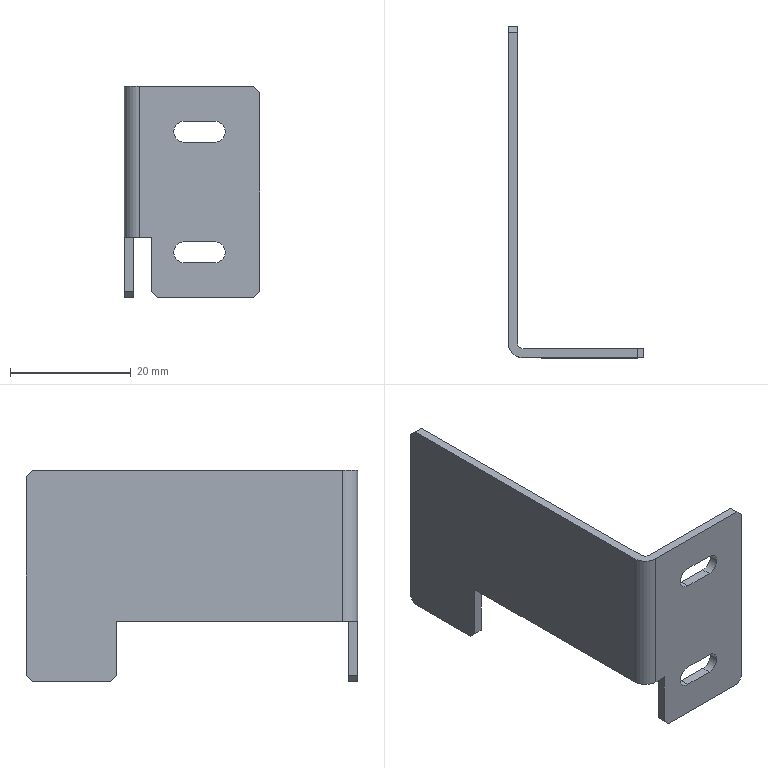Part | SolidWorks | features BaseBody 1 | 1 solid | 28 faces | box 22.5 x 55 x 35 mm | volume 3231 mm3 | plane 22 | cylinder 6 | commonest cylinder face diameters 3.5 x4 2 x1 5 x1
STEP:
#1=CARTESIAN_POINT('',(9.,-1.5,-17.5));
#2=VERTEX_POINT('',#1);
#3=CARTESIAN_POINT('',(10.,-1.5,-16.5));
#4=VERTEX_POINT('',#3);
#5=CARTESIAN_POINT('',(10.,-1.5,-16.5));
#6=DIRECTION('',(0.7071,0.,0.7071));
#7=VECTOR('',#6,1000.);
#8=LINE('',#5,#7);
#9=EDGE_CURVE('',#2,#4,#8,.T.);
#10=ORIENTED_EDGE('',*,*,#9,.F.);
#11=CARTESIAN_POINT('',(9.,0.,-17.5));
#12=VERTEX_POINT('',#11);
#13=CARTESIAN_POINT('',(9.,-1.5,-17.5));
#14=DIRECTION('',(0.,-1.,0.));
#15=VECTOR('',#14,1000.);
#16=LINE('',#13,#15);
#17=EDGE_CURVE('',#12,#2,#16,.T.);
#18=ORIENTED_EDGE('',*,*,#17,.F.);
#19=CARTESIAN_POINT('',(10.,0.,-16.5));
#20=VERTEX_POINT('',#19);
#21=CARTESIAN_POINT('',(13.25,0.,-13.25));
#22=DIRECTION('',(-0.7071,0.,-0.7071));
#23=VECTOR('',#22,1000.);
#24=LINE('',#21,#23);
#25=EDGE_CURVE('',#20,#12,#24,.T.);
#26=ORIENTED_EDGE('',*,*,#25,.F.);
#27=CARTESIAN_POINT('',(10.,-1.5,-16.5));
#28=DIRECTION('',(0.,1.,0.));
#29=VECTOR('',#28,1000.);
#30=LINE('',#27,#29);
#31=EDGE_CURVE('',#4,#20,#30,.T.);
#32=ORIENTED_EDGE('',*,*,#31,.F.);
#33=EDGE_LOOP('',(#10,#18,#26,#32));
#34=FACE_OUTER_BOUND('',#33,.T.);
#35=CARTESIAN_POINT('',(10.,-1.5,-16.5));
#36=DIRECTION('',(-0.7071,0.,0.7071));
#37=DIRECTION('',(0.,1.,0.));
#38=AXIS2_PLACEMENT_3D('',#35,#36,#37);
#39=PLANE('',#38);
#40=ADVANCED_FACE('',(#34),#39,.F.);
#41=CARTESIAN_POINT('',(10.,-1.5,16.5));
#42=VERTEX_POINT('',#41);
#43=CARTESIAN_POINT('',(9.,-1.5,17.5));
#44=VERTEX_POINT('',#43);
#45=CARTESIAN_POINT('',(9.,-1.5,17.5));
#46=DIRECTION('',(-0.7071,0.,0.7071));
#47=VECTOR('',#46,1000.);
#48=LINE('',#45,#47);
#49=EDGE_CURVE('',#42,#44,#48,.T.);
#50=ORIENTED_EDGE('',*,*,#49,.F.);
#51=CARTESIAN_POINT('',(10.,0.,16.5));
#52=VERTEX_POINT('',#51);
#53=CARTESIAN_POINT('',(10.,-1.5,16.5));
#54=DIRECTION('',(0.,-1.,0.));
#55=VECTOR('',#54,1000.);
#56=LINE('',#53,#55);
#57=EDGE_CURVE('',#52,#42,#56,.T.);
#58=ORIENTED_EDGE('',*,*,#57,.F.);
#59=CARTESIAN_POINT('',(9.,0.,17.5));
#60=VERTEX_POINT('',#59);
#61=CARTESIAN_POINT('',(13.25,0.,13.25));
#62=DIRECTION('',(0.7071,0.,-0.7071));
#63=VECTOR('',#62,1000.);
#64=LINE('',#61,#63);
#65=EDGE_CURVE('',#60,#52,#64,.T.);
#66=ORIENTED_EDGE('',*,*,#65,.F.);
#67=CARTESIAN_POINT('',(9.,-1.5,17.5));
#68=DIRECTION('',(0.,1.,0.));
#69=VECTOR('',#68,1000.);
#70=LINE('',#67,#69);
#71=EDGE_CURVE('',#44,#60,#70,.T.);
#72=ORIENTED_EDGE('',*,*,#71,.F.);
#73=EDGE_LOOP('',(#50,#58,#66,#72));
#74=FACE_OUTER_BOUND('',#73,.T.);
#75=CARTESIAN_POINT('',(9.,-1.5,17.5));
#76=DIRECTION('',(-0.7071,0.,-0.7071));
#77=DIRECTION('',(-0.7071,0.,0.7071));
#78=AXIS2_PLACEMENT_3D('',#75,#76,#77);
#79=PLANE('',#78);
#80=ADVANCED_FACE('',(#74),#79,.F.);
#81=CARTESIAN_POINT('',(-8.,-1.5,-16.5));
#82=VERTEX_POINT('',#81);
#83=CARTESIAN_POINT('',(-7.,-1.5,-17.5));
#84=VERTEX_POINT('',#83);
#85=CARTESIAN_POINT('',(-7.,-1.5,-17.5));
#86=DIRECTION('',(0.7071,0.,-0.7071));
#87=VECTOR('',#86,1000.);
#88=LINE('',#85,#87);
#89=EDGE_CURVE('',#82,#84,#88,.T.);
#90=ORIENTED_EDGE('',*,*,#89,.F.);
#91=CARTESIAN_POINT('',(-8.,0.,-16.5));
#92=VERTEX_POINT('',#91);
#93=CARTESIAN_POINT('',(-8.,0.,-16.5));
#94=DIRECTION('',(0.,-1.,0.));
#95=VECTOR('',#94,1000.);
#96=LINE('',#93,#95);
#97=EDGE_CURVE('',#92,#82,#96,.T.);
#98=ORIENTED_EDGE('',*,*,#97,.F.);
#99=CARTESIAN_POINT('',(-7.,0.,-17.5));
#100=VERTEX_POINT('',#99);
#101=CARTESIAN_POINT('',(-12.25,0.,-12.25));
#102=DIRECTION('',(-0.7071,0.,0.7071));
#103=VECTOR('',#102,1000.);
#104=LINE('',#101,#103);
#105=EDGE_CURVE('',#100,#92,#104,.T.);
#106=ORIENTED_EDGE('',*,*,#105,.F.);
#107=CARTESIAN_POINT('',(-7.,-1.5,-17.5));
#108=DIRECTION('',(0.,1.,0.));
#109=VECTOR('',#108,1000.);
#110=LINE('',#107,#109);
#111=EDGE_CURVE('',#84,#100,#110,.T.);
#112=ORIENTED_EDGE('',*,*,#111,.F.);
#113=EDGE_LOOP('',(#90,#98,#106,#112));
#114=FACE_OUTER_BOUND('',#113,.T.);
#115=CARTESIAN_POINT('',(-7.,-1.5,-17.5));
#116=DIRECTION('',(0.7071,0.,0.7071));
#117=DIRECTION('',(0.,-1.,0.));
#118=AXIS2_PLACEMENT_3D('',#115,#116,#117);
#119=PLANE('',#118);
#120=ADVANCED_FACE('',(#114),#119,.F.);
#121=CARTESIAN_POINT('',(-12.5,53.5,-16.5));
#122=VERTEX_POINT('',#121);
#123=CARTESIAN_POINT('',(-12.5,52.5,-17.5));
#124=VERTEX_POINT('',#123);
#125=CARTESIAN_POINT('',(-12.5,52.5,-17.5));
#126=DIRECTION('',(0.,-0.7071,-0.7071));
#127=VECTOR('',#126,1000.);
#128=LINE('',#125,#127);
#129=EDGE_CURVE('',#122,#124,#128,.T.);
#130=ORIENTED_EDGE('',*,*,#129,.F.);
#131=CARTESIAN_POINT('',(-11.,53.5,-16.5));
#132=VERTEX_POINT('',#131);
#133=CARTESIAN_POINT('',(-12.5,53.5,-16.5));
#134=DIRECTION('',(-1.,0.,0.));
#135=VECTOR('',#134,1000.);
#136=LINE('',#133,#135);
#137=EDGE_CURVE('',#132,#122,#136,.T.);
#138=ORIENTED_EDGE('',*,*,#137,.F.);
#139=CARTESIAN_POINT('',(-11.,52.5,-17.5));
#140=VERTEX_POINT('',#139);
#141=CARTESIAN_POINT('',(-11.,35.,-35.));
#142=DIRECTION('',(0.,0.7071,0.7071));
#143=VECTOR('',#142,1000.);
#144=LINE('',#141,#143);
#145=EDGE_CURVE('',#140,#132,#144,.T.);
#146=ORIENTED_EDGE('',*,*,#145,.F.);
#147=CARTESIAN_POINT('',(-12.5,52.5,-17.5));
#148=DIRECTION('',(1.,0.,0.));
#149=VECTOR('',#148,1000.);
#150=LINE('',#147,#149);
#151=EDGE_CURVE('',#124,#140,#150,.T.);
#152=ORIENTED_EDGE('',*,*,#151,.F.);
#153=EDGE_LOOP('',(#130,#138,#146,#152));
#154=FACE_OUTER_BOUND('',#153,.T.);
#155=CARTESIAN_POINT('',(-12.5,52.5,-17.5));
#156=DIRECTION('',(0.,-0.7071,0.7071));
#157=DIRECTION('',(-1.,0.,0.));
#158=AXIS2_PLACEMENT_3D('',#155,#156,#157);
#159=PLANE('',#158);
#160=ADVANCED_FACE('',(#154),#159,.F.);
#161=CARTESIAN_POINT('',(-12.5,39.5,-17.5));
#162=VERTEX_POINT('',#161);
#163=CARTESIAN_POINT('',(-12.5,38.5,-16.5));
#164=VERTEX_POINT('',#163);
#165=CARTESIAN_POINT('',(-12.5,38.5,-16.5));
#166=DIRECTION('',(0.,-0.7071,0.7071));
#167=VECTOR('',#166,1000.);
#168=LINE('',#165,#167);
#169=EDGE_CURVE('',#162,#164,#168,.T.);
#170=ORIENTED_EDGE('',*,*,#169,.F.);
#171=CARTESIAN_POINT('',(-11.,39.5,-17.5));
#172=VERTEX_POINT('',#171);
#173=CARTESIAN_POINT('',(-12.5,39.5,-17.5));
#174=DIRECTION('',(-1.,0.,0.));
#175=VECTOR('',#174,1000.);
#176=LINE('',#173,#175);
#177=EDGE_CURVE('',#172,#162,#176,.T.);
#178=ORIENTED_EDGE('',*,*,#177,.F.);
#179=CARTESIAN_POINT('',(-11.,38.5,-16.5));
#180=VERTEX_POINT('',#179);
#181=CARTESIAN_POINT('',(-11.,11.,11.));
#182=DIRECTION('',(0.,0.7071,-0.7071));
#183=VECTOR('',#182,1000.);
#184=LINE('',#181,#183);
#185=EDGE_CURVE('',#180,#172,#184,.T.);
#186=ORIENTED_EDGE('',*,*,#185,.F.);
#187=CARTESIAN_POINT('',(-14.,38.5,-16.5));
#188=DIRECTION('',(1.,0.,0.));
#189=VECTOR('',#188,1000.);
#190=LINE('',#187,#189);
#191=EDGE_CURVE('',#164,#180,#190,.T.);
#192=ORIENTED_EDGE('',*,*,#191,.F.);
#193=EDGE_LOOP('',(#170,#178,#186,#192));
#194=FACE_OUTER_BOUND('',#193,.T.);
#195=CARTESIAN_POINT('',(-14.,38.5,-16.5));
#196=DIRECTION('',(0.,0.7071,0.7071));
#197=DIRECTION('',(1.,0.,0.));
#198=AXIS2_PLACEMENT_3D('',#195,#196,#197);
#199=PLANE('',#198);
#200=ADVANCED_FACE('',(#194),#199,.F.);
#201=CARTESIAN_POINT('',(-12.5,52.5,17.5));
#202=VERTEX_POINT('',#201);
#203=CARTESIAN_POINT('',(-12.5,53.5,16.5));
#204=VERTEX_POINT('',#203);
#205=CARTESIAN_POINT('',(-12.5,53.5,16.5));
#206=DIRECTION('',(0.,0.7071,-0.7071));
#207=VECTOR('',#206,1000.);
#208=LINE('',#205,#207);
#209=EDGE_CURVE('',#202,#204,#208,.T.);
#210=ORIENTED_EDGE('',*,*,#209,.F.);
#211=CARTESIAN_POINT('',(-11.,52.5,17.5));
#212=VERTEX_POINT('',#211);
#213=CARTESIAN_POINT('',(-12.5,52.5,17.5));
#214=DIRECTION('',(-1.,0.,0.));
#215=VECTOR('',#214,1000.);
#216=LINE('',#213,#215);
#217=EDGE_CURVE('',#212,#202,#216,.T.);
#218=ORIENTED_EDGE('',*,*,#217,.F.);
#219=CARTESIAN_POINT('',(-11.,53.5,16.5));
#220=VERTEX_POINT('',#219);
#221=CARTESIAN_POINT('',(-11.,35.,35.));
#222=DIRECTION('',(0.,-0.7071,0.7071));
#223=VECTOR('',#222,1000.);
#224=LINE('',#221,#223);
#225=EDGE_CURVE('',#220,#212,#224,.T.);
#226=ORIENTED_EDGE('',*,*,#225,.F.);
#227=CARTESIAN_POINT('',(-12.5,53.5,16.5));
#228=DIRECTION('',(1.,0.,0.));
#229=VECTOR('',#228,1000.);
#230=LINE('',#227,#229);
#231=EDGE_CURVE('',#204,#220,#230,.T.);
#232=ORIENTED_EDGE('',*,*,#231,.F.);
#233=EDGE_LOOP('',(#210,#218,#226,#232));
#234=FACE_OUTER_BOUND('',#233,.T.);
#235=CARTESIAN_POINT('',(-12.5,53.5,16.5));
#236=DIRECTION('',(0.,-0.7071,-0.7071));
#237=DIRECTION('',(0.,-0.7071,0.7071));
#238=AXIS2_PLACEMENT_3D('',#235,#236,#237);
#239=PLANE('',#238);
#240=ADVANCED_FACE('',(#234),#239,.F.);
#241=CARTESIAN_POINT('',(-12.5,38.5,-7.5));
#242=VERTEX_POINT('',#241);
#243=CARTESIAN_POINT('',(-12.5,38.5,0.));
#244=DIRECTION('',(0.,0.,1.));
#245=VECTOR('',#244,1000.);
#246=LINE('',#243,#245);
#247=EDGE_CURVE('',#164,#242,#246,.T.);
#248=ORIENTED_EDGE('',*,*,#247,.F.);
#249=ORIENTED_EDGE('',*,*,#191,.T.);
#250=CARTESIAN_POINT('',(-11.,38.5,-7.5));
#251=VERTEX_POINT('',#250);
#252=CARTESIAN_POINT('',(-11.,38.5,0.));
#253=DIRECTION('',(0.,0.,1.));
#254=VECTOR('',#253,1000.);
#255=LINE('',#252,#254);
#256=EDGE_CURVE('',#180,#251,#255,.T.);
#257=ORIENTED_EDGE('',*,*,#256,.T.);
#258=CARTESIAN_POINT('',(-14.,38.5,-7.5));
#259=DIRECTION('',(1.,0.,0.));
#260=VECTOR('',#259,1000.);
#261=LINE('',#258,#260);
#262=EDGE_CURVE('',#242,#251,#261,.T.);
#263=ORIENTED_EDGE('',*,*,#262,.F.);
#264=EDGE_LOOP('',(#248,#249,#257,#263));
#265=FACE_OUTER_BOUND('',#264,.T.);
#266=CARTESIAN_POINT('',(-14.,38.5,-17.5));
#267=DIRECTION('',(0.,1.,0.));
#268=DIRECTION('',(1.,0.,0.));
#269=AXIS2_PLACEMENT_3D('',#266,#267,#268);
#270=PLANE('',#269);
#271=ADVANCED_FACE('',(#265),#270,.F.);
#272=CARTESIAN_POINT('',(-10.,-1.5,-7.5));
#273=VERTEX_POINT('',#272);
#274=CARTESIAN_POINT('',(-12.5,1.,-7.5));
#275=VERTEX_POINT('',#274);
#276=CARTESIAN_POINT('',(-10.,1.,-7.5));
#277=DIRECTION('',(0.,0.,-1.));
#278=DIRECTION('',(0.,-1.,0.));
#279=AXIS2_PLACEMENT_3D('',#276,#277,#278);
#280=CIRCLE('',#279,2.5);
#281=EDGE_CURVE('',#273,#275,#280,.T.);
#282=ORIENTED_EDGE('',*,*,#281,.T.);
#283=CARTESIAN_POINT('',(-12.5,0.,-7.5));
#284=DIRECTION('',(0.,-1.,0.));
#285=VECTOR('',#284,1000.);
#286=LINE('',#283,#285);
#287=EDGE_CURVE('',#242,#275,#286,.T.);
#288=ORIENTED_EDGE('',*,*,#287,.F.);
#289=ORIENTED_EDGE('',*,*,#262,.T.);
#290=CARTESIAN_POINT('',(-11.,1.,-7.5));
#291=VERTEX_POINT('',#290);
#292=CARTESIAN_POINT('',(-11.,0.,-7.5));
#293=DIRECTION('',(0.,-1.,0.));
#294=VECTOR('',#293,1000.);
#295=LINE('',#292,#294);
#296=EDGE_CURVE('',#251,#291,#295,.T.);
#297=ORIENTED_EDGE('',*,*,#296,.T.);
#298=CARTESIAN_POINT('',(-10.,0.,-7.5));
#299=VERTEX_POINT('',#298);
#300=CARTESIAN_POINT('',(-10.,1.,-7.5));
#301=DIRECTION('',(0.,0.,-1.));
#302=DIRECTION('',(0.,-1.,0.));
#303=AXIS2_PLACEMENT_3D('',#300,#301,#302);
#304=CIRCLE('',#303,1.);
#305=EDGE_CURVE('',#299,#291,#304,.T.);
#306=ORIENTED_EDGE('',*,*,#305,.F.);
#307=CARTESIAN_POINT('',(-8.,0.,-7.5));
#308=VERTEX_POINT('',#307);
#309=CARTESIAN_POINT('',(0.,0.,-7.5));
#310=DIRECTION('',(1.,0.,0.));
#311=VECTOR('',#310,1000.);
#312=LINE('',#309,#311);
#313=EDGE_CURVE('',#299,#308,#312,.T.);
#314=ORIENTED_EDGE('',*,*,#313,.T.);
#315=CARTESIAN_POINT('',(-8.,-1.5,-7.5));
#316=VERTEX_POINT('',#315);
#317=CARTESIAN_POINT('',(-8.,38.5,-7.5));
#318=DIRECTION('',(0.,-1.,0.));
#319=VECTOR('',#318,1000.);
#320=LINE('',#317,#319);
#321=EDGE_CURVE('',#308,#316,#320,.T.);
#322=ORIENTED_EDGE('',*,*,#321,.T.);
#323=CARTESIAN_POINT('',(0.,-1.5,-7.5));
#324=DIRECTION('',(1.,0.,0.));
#325=VECTOR('',#324,1000.);
#326=LINE('',#323,#325);
#327=EDGE_CURVE('',#273,#316,#326,.T.);
#328=ORIENTED_EDGE('',*,*,#327,.F.);
#329=EDGE_LOOP('',(#282,#288,#289,#297,#306,#314,#322,#328));
#330=FACE_OUTER_BOUND('',#329,.T.);
#331=CARTESIAN_POINT('',(-14.,38.5,-7.5));
#332=DIRECTION('',(0.,0.,1.));
#333=DIRECTION('',(0.,-1.,0.));
#334=AXIS2_PLACEMENT_3D('',#331,#332,#333);
#335=PLANE('',#334);
#336=ADVANCED_FACE('',(#330),#335,.F.);
#337=CARTESIAN_POINT('',(-8.,0.,0.));
#338=DIRECTION('',(0.,0.,1.));
#339=VECTOR('',#338,1000.);
#340=LINE('',#337,#339);
#341=EDGE_CURVE('',#92,#308,#340,.T.);
#342=ORIENTED_EDGE('',*,*,#341,.F.);
#343=ORIENTED_EDGE('',*,*,#97,.T.);
#344=CARTESIAN_POINT('',(-8.,-1.5,0.));
#345=DIRECTION('',(0.,0.,1.));
#346=VECTOR('',#345,1000.);
#347=LINE('',#344,#346);
#348=EDGE_CURVE('',#82,#316,#347,.T.);
#349=ORIENTED_EDGE('',*,*,#348,.T.);
#350=ORIENTED_EDGE('',*,*,#321,.F.);
#351=EDGE_LOOP('',(#342,#343,#349,#350));
#352=FACE_OUTER_BOUND('',#351,.T.);
#353=CARTESIAN_POINT('',(-8.,0.,0.));
#354=DIRECTION('',(-1.,0.,0.));
#355=DIRECTION('',(0.,1.,0.));
#356=AXIS2_PLACEMENT_3D('',#353,#354,#355);
#357=PLANE('',#356);
#358=ADVANCED_FACE('',(#352),#357,.T.);
#359=CARTESIAN_POINT('',(2.5,0.,11.75));
#360=VERTEX_POINT('',#359);
#361=CARTESIAN_POINT('',(2.5,0.,8.25));
#362=VERTEX_POINT('',#361);
#363=CARTESIAN_POINT('',(2.5,0.,10.));
#364=DIRECTION('',(0.,1.,0.));
#365=DIRECTION('',(0.,0.,1.));
#366=AXIS2_PLACEMENT_3D('',#363,#364,#365);
#367=CIRCLE('',#366,1.75);
#368=EDGE_CURVE('',#360,#362,#367,.T.);
#369=ORIENTED_EDGE('',*,*,#368,.T.);
#370=CARTESIAN_POINT('',(2.5,-1.5,8.25));
#371=VERTEX_POINT('',#370);
#372=CARTESIAN_POINT('',(2.5,8.5,8.25));
#373=DIRECTION('',(0.,-1.,0.));
#374=VECTOR('',#373,1000.);
#375=LINE('',#372,#374);
#376=EDGE_CURVE('',#362,#371,#375,.T.);
#377=ORIENTED_EDGE('',*,*,#376,.T.);
#378=CARTESIAN_POINT('',(2.5,-1.5,11.75));
#379=VERTEX_POINT('',#378);
#380=CARTESIAN_POINT('',(2.5,-1.5,10.));
#381=DIRECTION('',(0.,-1.,0.));
#382=DIRECTION('',(0.,0.,-1.));
#383=AXIS2_PLACEMENT_3D('',#380,#381,#382);
#384=CIRCLE('',#383,1.75);
#385=EDGE_CURVE('',#371,#379,#384,.T.);
#386=ORIENTED_EDGE('',*,*,#385,.T.);
#387=CARTESIAN_POINT('',(2.5,8.5,11.75));
#388=DIRECTION('',(0.,-1.,0.));
#389=VECTOR('',#388,1000.);
#390=LINE('',#387,#389);
#391=EDGE_CURVE('',#360,#379,#390,.T.);
#392=ORIENTED_EDGE('',*,*,#391,.F.);
#393=EDGE_LOOP('',(#369,#377,#386,#392));
#394=FACE_OUTER_BOUND('',#393,.T.);
#395=CARTESIAN_POINT('',(2.5,8.5,10.));
#396=DIRECTION('',(0.,-1.,0.));
#397=DIRECTION('',(0.,0.,-1.));
#398=AXIS2_PLACEMENT_3D('',#395,#396,#397);
#399=CYLINDRICAL_SURFACE('',#398,1.75);
#400=ADVANCED_FACE('',(#394),#399,.F.);
#401=CARTESIAN_POINT('',(-2.5,0.,8.25));
#402=VERTEX_POINT('',#401);
#403=CARTESIAN_POINT('',(-2.5,0.,11.75));
#404=VERTEX_POINT('',#403);
#405=CARTESIAN_POINT('',(-2.5,0.,10.));
#406=DIRECTION('',(0.,1.,0.));
#407=DIRECTION('',(0.,0.,1.));
#408=AXIS2_PLACEMENT_3D('',#405,#406,#407);
#409=CIRCLE('',#408,1.75);
#410=EDGE_CURVE('',#402,#404,#409,.T.);
#411=ORIENTED_EDGE('',*,*,#410,.T.);
#412=CARTESIAN_POINT('',(-2.5,-1.5,11.75));
#413=VERTEX_POINT('',#412);
#414=CARTESIAN_POINT('',(-2.5,8.5,11.75));
#415=DIRECTION('',(0.,-1.,0.));
#416=VECTOR('',#415,1000.);
#417=LINE('',#414,#416);
#418=EDGE_CURVE('',#404,#413,#417,.T.);
#419=ORIENTED_EDGE('',*,*,#418,.T.);
#420=CARTESIAN_POINT('',(-2.5,-1.5,8.25));
#421=VERTEX_POINT('',#420);
#422=CARTESIAN_POINT('',(-2.5,-1.5,10.));
#423=DIRECTION('',(0.,-1.,0.));
#424=DIRECTION('',(0.,0.,-1.));
#425=AXIS2_PLACEMENT_3D('',#422,#423,#424);
#426=CIRCLE('',#425,1.75);
#427=EDGE_CURVE('',#413,#421,#426,.T.);
#428=ORIENTED_EDGE('',*,*,#427,.T.);
#429=CARTESIAN_POINT('',(-2.5,8.5,8.25));
#430=DIRECTION('',(0.,-1.,0.));
#431=VECTOR('',#430,1000.);
#432=LINE('',#429,#431);
#433=EDGE_CURVE('',#402,#421,#432,.T.);
#434=ORIENTED_EDGE('',*,*,#433,.F.);
#435=EDGE_LOOP('',(#411,#419,#428,#434));
#436=FACE_OUTER_BOUND('',#435,.T.);
#437=CARTESIAN_POINT('',(-2.5,8.5,10.));
#438=DIRECTION('',(0.,-1.,0.));
#439=DIRECTION('',(0.,0.,-1.));
#440=AXIS2_PLACEMENT_3D('',#437,#438,#439);
#441=CYLINDRICAL_SURFACE('',#440,1.75);
#442=ADVANCED_FACE('',(#436),#441,.F.);
#443=CARTESIAN_POINT('',(0.,0.,8.25));
#444=DIRECTION('',(-1.,0.,0.));
#445=VECTOR('',#444,1000.);
#446=LINE('',#443,#445);
#447=EDGE_CURVE('',#362,#402,#446,.T.);
#448=ORIENTED_EDGE('',*,*,#447,.T.);
#449=ORIENTED_EDGE('',*,*,#433,.T.);
#450=CARTESIAN_POINT('',(-2.5,-1.5,8.25));
#451=DIRECTION('',(1.,0.,0.));
#452=VECTOR('',#451,1000.);
#453=LINE('',#450,#452);
#454=EDGE_CURVE('',#421,#371,#453,.T.);
#455=ORIENTED_EDGE('',*,*,#454,.T.);
#456=ORIENTED_EDGE('',*,*,#376,.F.);
#457=EDGE_LOOP('',(#448,#449,#455,#456));
#458=FACE_OUTER_BOUND('',#457,.T.);
#459=CARTESIAN_POINT('',(-2.5,8.5,8.25));
#460=DIRECTION('',(0.,0.,-1.));
#461=DIRECTION('',(0.,-1.,0.));
#462=AXIS2_PLACEMENT_3D('',#459,#460,#461);
#463=PLANE('',#462);
#464=ADVANCED_FACE('',(#458),#463,.F.);
#465=CARTESIAN_POINT('',(0.,0.,11.75));
#466=DIRECTION('',(1.,0.,0.));
#467=VECTOR('',#466,1000.);
#468=LINE('',#465,#467);
#469=EDGE_CURVE('',#404,#360,#468,.T.);
#470=ORIENTED_EDGE('',*,*,#469,.T.);
#471=ORIENTED_EDGE('',*,*,#391,.T.);
#472=CARTESIAN_POINT('',(-2.5,-1.5,11.75));
#473=DIRECTION('',(-1.,0.,0.));
#474=VECTOR('',#473,1000.);
#475=LINE('',#472,#474);
#476=EDGE_CURVE('',#379,#413,#475,.T.);
#477=ORIENTED_EDGE('',*,*,#476,.T.);
#478=ORIENTED_EDGE('',*,*,#418,.F.);
#479=EDGE_LOOP('',(#470,#471,#477,#478));
#480=FACE_OUTER_BOUND('',#479,.T.);
#481=CARTESIAN_POINT('',(-2.5,8.5,11.75));
#482=DIRECTION('',(0.,0.,1.));
#483=DIRECTION('',(1.,0.,0.));
#484=AXIS2_PLACEMENT_3D('',#481,#482,#483);
#485=PLANE('',#484);
#486=ADVANCED_FACE('',(#480),#485,.F.);
#487=CARTESIAN_POINT('',(2.5,0.,-8.25));
#488=VERTEX_POINT('',#487);
#489=CARTESIAN_POINT('',(2.5,0.,-11.75));
#490=VERTEX_POINT('',#489);
#491=CARTESIAN_POINT('',(2.5,0.,-10.));
#492=DIRECTION('',(0.,1.,0.));
#493=DIRECTION('',(0.,0.,1.));
#494=AXIS2_PLACEMENT_3D('',#491,#492,#493);
#495=CIRCLE('',#494,1.75);
#496=EDGE_CURVE('',#488,#490,#495,.T.);
#497=ORIENTED_EDGE('',*,*,#496,.T.);
#498=CARTESIAN_POINT('',(2.5,-1.5,-11.75));
#499=VERTEX_POINT('',#498);
#500=CARTESIAN_POINT('',(2.5,8.5,-11.75));
#501=DIRECTION('',(0.,-1.,0.));
#502=VECTOR('',#501,1000.);
#503=LINE('',#500,#502);
#504=EDGE_CURVE('',#490,#499,#503,.T.);
#505=ORIENTED_EDGE('',*,*,#504,.T.);
#506=CARTESIAN_POINT('',(2.5,-1.5,-8.25));
#507=VERTEX_POINT('',#506);
#508=CARTESIAN_POINT('',(2.5,-1.5,-10.));
#509=DIRECTION('',(0.,-1.,0.));
#510=DIRECTION('',(0.,0.,-1.));
#511=AXIS2_PLACEMENT_3D('',#508,#509,#510);
#512=CIRCLE('',#511,1.75);
#513=EDGE_CURVE('',#499,#507,#512,.T.);
#514=ORIENTED_EDGE('',*,*,#513,.T.);
#515=CARTESIAN_POINT('',(2.5,8.5,-8.25));
#516=DIRECTION('',(0.,-1.,0.));
#517=VECTOR('',#516,1000.);
#518=LINE('',#515,#517);
#519=EDGE_CURVE('',#488,#507,#518,.T.);
#520=ORIENTED_EDGE('',*,*,#519,.F.);
#521=EDGE_LOOP('',(#497,#505,#514,#520));
#522=FACE_OUTER_BOUND('',#521,.T.);
#523=CARTESIAN_POINT('',(2.5,8.5,-10.));
#524=DIRECTION('',(0.,-1.,0.));
#525=DIRECTION('',(0.,0.,-1.));
#526=AXIS2_PLACEMENT_3D('',#523,#524,#525);
#527=CYLINDRICAL_SURFACE('',#526,1.75);
#528=ADVANCED_FACE('',(#522),#527,.F.);
#529=CARTESIAN_POINT('',(-2.5,0.,-11.75));
#530=VERTEX_POINT('',#529);
#531=CARTESIAN_POINT('',(-2.5,0.,-8.25));
#532=VERTEX_POINT('',#531);
#533=CARTESIAN_POINT('',(-2.5,0.,-10.));
#534=DIRECTION('',(0.,1.,0.));
#535=DIRECTION('',(0.,0.,1.));
#536=AXIS2_PLACEMENT_3D('',#533,#534,#535);
#537=CIRCLE('',#536,1.75);
#538=EDGE_CURVE('',#530,#532,#537,.T.);
#539=ORIENTED_EDGE('',*,*,#538,.T.);
#540=CARTESIAN_POINT('',(-2.5,-1.5,-8.25));
#541=VERTEX_POINT('',#540);
#542=CARTESIAN_POINT('',(-2.5,8.5,-8.25));
#543=DIRECTION('',(0.,-1.,0.));
#544=VECTOR('',#543,1000.);
#545=LINE('',#542,#544);
#546=EDGE_CURVE('',#532,#541,#545,.T.);
#547=ORIENTED_EDGE('',*,*,#546,.T.);
#548=CARTESIAN_POINT('',(-2.5,-1.5,-11.75));
#549=VERTEX_POINT('',#548);
#550=CARTESIAN_POINT('',(-2.5,-1.5,-10.));
#551=DIRECTION('',(0.,-1.,0.));
#552=DIRECTION('',(0.,0.,-1.));
#553=AXIS2_PLACEMENT_3D('',#550,#551,#552);
#554=CIRCLE('',#553,1.75);
#555=EDGE_CURVE('',#541,#549,#554,.T.);
#556=ORIENTED_EDGE('',*,*,#555,.T.);
#557=CARTESIAN_POINT('',(-2.5,8.5,-11.75));
#558=DIRECTION('',(0.,-1.,0.));
#559=VECTOR('',#558,1000.);
#560=LINE('',#557,#559);
#561=EDGE_CURVE('',#530,#549,#560,.T.);
#562=ORIENTED_EDGE('',*,*,#561,.F.);
#563=EDGE_LOOP('',(#539,#547,#556,#562));
#564=FACE_OUTER_BOUND('',#563,.T.);
#565=CARTESIAN_POINT('',(-2.5,8.5,-10.));
#566=DIRECTION('',(0.,-1.,0.));
#567=DIRECTION('',(0.,0.,-1.));
#568=AXIS2_PLACEMENT_3D('',#565,#566,#567);
#569=CYLINDRICAL_SURFACE('',#568,1.75);
#570=ADVANCED_FACE('',(#564),#569,.F.);
#571=CARTESIAN_POINT('',(0.,0.,-11.75));
#572=DIRECTION('',(-1.,0.,0.));
#573=VECTOR('',#572,1000.);
#574=LINE('',#571,#573);
#575=EDGE_CURVE('',#490,#530,#574,.T.);
#576=ORIENTED_EDGE('',*,*,#575,.T.);
#577=ORIENTED_EDGE('',*,*,#561,.T.);
#578=CARTESIAN_POINT('',(-2.5,-1.5,-11.75));
#579=DIRECTION('',(1.,0.,0.));
#580=VECTOR('',#579,1000.);
#581=LINE('',#578,#580);
#582=EDGE_CURVE('',#549,#499,#581,.T.);
#583=ORIENTED_EDGE('',*,*,#582,.T.);
#584=ORIENTED_EDGE('',*,*,#504,.F.);
#585=EDGE_LOOP('',(#576,#577,#583,#584));
#586=FACE_OUTER_BOUND('',#585,.T.);
#587=CARTESIAN_POINT('',(-2.5,8.5,-11.75));
#588=DIRECTION('',(0.,0.,-1.));
#589=DIRECTION('',(0.,-1.,0.));
#590=AXIS2_PLACEMENT_3D('',#587,#588,#589);
#591=PLANE('',#590);
#592=ADVANCED_FACE('',(#586),#591,.F.);
#593=CARTESIAN_POINT('',(0.,0.,-8.25));
#594=DIRECTION('',(1.,0.,0.));
#595=VECTOR('',#594,1000.);
#596=LINE('',#593,#595);
#597=EDGE_CURVE('',#532,#488,#596,.T.);
#598=ORIENTED_EDGE('',*,*,#597,.T.);
#599=ORIENTED_EDGE('',*,*,#519,.T.);
#600=CARTESIAN_POINT('',(-2.5,-1.5,-8.25));
#601=DIRECTION('',(-1.,0.,0.));
#602=VECTOR('',#601,1000.);
#603=LINE('',#600,#602);
#604=EDGE_CURVE('',#507,#541,#603,.T.);
#605=ORIENTED_EDGE('',*,*,#604,.T.);
#606=ORIENTED_EDGE('',*,*,#546,.F.);
#607=EDGE_LOOP('',(#598,#599,#605,#606));
#608=FACE_OUTER_BOUND('',#607,.T.);
#609=CARTESIAN_POINT('',(-2.5,8.5,-8.25));
#610=DIRECTION('',(0.,0.,1.));
#611=DIRECTION('',(1.,0.,0.));
#612=AXIS2_PLACEMENT_3D('',#609,#610,#611);
#613=PLANE('',#612);
#614=ADVANCED_FACE('',(#608),#613,.F.);
#615=CARTESIAN_POINT('',(-12.5,53.5,0.));
#616=DIRECTION('',(0.,0.,-1.));
#617=VECTOR('',#616,1000.);
#618=LINE('',#615,#617);
#619=EDGE_CURVE('',#204,#122,#618,.T.);
#620=ORIENTED_EDGE('',*,*,#619,.F.);
#621=ORIENTED_EDGE('',*,*,#231,.T.);
#622=CARTESIAN_POINT('',(-11.,53.5,-17.5));
#623=DIRECTION('',(0.,0.,-1.));
#624=VECTOR('',#623,1000.);
#625=LINE('',#622,#624);
#626=EDGE_CURVE('',#220,#132,#625,.T.);
#627=ORIENTED_EDGE('',*,*,#626,.T.);
#628=ORIENTED_EDGE('',*,*,#137,.T.);
#629=EDGE_LOOP('',(#620,#621,#627,#628));
#630=FACE_OUTER_BOUND('',#629,.T.);
#631=CARTESIAN_POINT('',(-12.5,53.5,-17.5));
#632=DIRECTION('',(0.,-1.,0.));
#633=DIRECTION('',(0.,0.,-1.));
#634=AXIS2_PLACEMENT_3D('',#631,#632,#633);
#635=PLANE('',#634);
#636=ADVANCED_FACE('',(#630),#635,.F.);
#637=ORIENTED_EDGE('',*,*,#626,.F.);
#638=ORIENTED_EDGE('',*,*,#225,.T.);
#639=CARTESIAN_POINT('',(-11.,1.,17.5));
#640=VERTEX_POINT('',#639);
#641=CARTESIAN_POINT('',(-11.,53.5,17.5));
#642=DIRECTION('',(0.,1.,0.));
#643=VECTOR('',#642,1000.);
#644=LINE('',#641,#643);
#645=EDGE_CURVE('',#640,#212,#644,.T.);
#646=ORIENTED_EDGE('',*,*,#645,.F.);
#647=CARTESIAN_POINT('',(-11.,1.,-17.5));
#648=DIRECTION('',(0.,0.,1.));
#649=VECTOR('',#648,1000.);
#650=LINE('',#647,#649);
#651=EDGE_CURVE('',#291,#640,#650,.T.);
#652=ORIENTED_EDGE('',*,*,#651,.F.);
#653=ORIENTED_EDGE('',*,*,#296,.F.);
#654=ORIENTED_EDGE('',*,*,#256,.F.);
#655=ORIENTED_EDGE('',*,*,#185,.T.);
#656=CARTESIAN_POINT('',(-11.,0.,-17.5));
#657=DIRECTION('',(0.,-1.,0.));
#658=VECTOR('',#657,1000.);
#659=LINE('',#656,#658);
#660=EDGE_CURVE('',#140,#172,#659,.T.);
#661=ORIENTED_EDGE('',*,*,#660,.F.);
#662=ORIENTED_EDGE('',*,*,#145,.T.);
#663=EDGE_LOOP('',(#637,#638,#646,#652,#653,#654,#655,#661,#662));
#664=FACE_OUTER_BOUND('',#663,.T.);
#665=CARTESIAN_POINT('',(-11.,0.,0.));
#666=DIRECTION('',(1.,0.,0.));
#667=DIRECTION('',(0.,1.,0.));
#668=AXIS2_PLACEMENT_3D('',#665,#666,#667);
#669=PLANE('',#668);
#670=ADVANCED_FACE('',(#664),#669,.T.);
#671=CARTESIAN_POINT('',(-12.5,1.,17.5));
#672=VERTEX_POINT('',#671);
#673=CARTESIAN_POINT('',(-12.5,0.,17.5));
#674=DIRECTION('',(0.,1.,0.));
#675=VECTOR('',#674,1000.);
#676=LINE('',#673,#675);
#677=EDGE_CURVE('',#672,#202,#676,.T.);
#678=ORIENTED_EDGE('',*,*,#677,.T.);
#679=ORIENTED_EDGE('',*,*,#209,.T.);
#680=ORIENTED_EDGE('',*,*,#619,.T.);
#681=ORIENTED_EDGE('',*,*,#129,.T.);
#682=CARTESIAN_POINT('',(-12.5,0.,-17.5));
#683=DIRECTION('',(0.,-1.,0.));
#684=VECTOR('',#683,1000.);
#685=LINE('',#682,#684);
#686=EDGE_CURVE('',#124,#162,#685,.T.);
#687=ORIENTED_EDGE('',*,*,#686,.T.);
#688=ORIENTED_EDGE('',*,*,#169,.T.);
#689=ORIENTED_EDGE('',*,*,#247,.T.);
#690=ORIENTED_EDGE('',*,*,#287,.T.);
#691=CARTESIAN_POINT('',(-12.5,1.,-17.5));
#692=DIRECTION('',(0.,0.,-1.));
#693=VECTOR('',#692,1000.);
#694=LINE('',#691,#693);
#695=EDGE_CURVE('',#672,#275,#694,.T.);
#696=ORIENTED_EDGE('',*,*,#695,.F.);
#697=EDGE_LOOP('',(#678,#679,#680,#681,#687,#688,#689,#690,#696));
#698=FACE_OUTER_BOUND('',#697,.T.);
#699=CARTESIAN_POINT('',(-12.5,0.,0.));
#700=DIRECTION('',(1.,0.,0.));
#701=DIRECTION('',(0.,1.,0.));
#702=AXIS2_PLACEMENT_3D('',#699,#700,#701);
#703=PLANE('',#702);
#704=ADVANCED_FACE('',(#698),#703,.F.);
#705=ORIENTED_EDGE('',*,*,#660,.T.);
#706=ORIENTED_EDGE('',*,*,#177,.T.);
#707=ORIENTED_EDGE('',*,*,#686,.F.);
#708=ORIENTED_EDGE('',*,*,#151,.T.);
#709=EDGE_LOOP('',(#705,#706,#707,#708));
#710=FACE_OUTER_BOUND('',#709,.T.);
#711=CARTESIAN_POINT('',(-12.5,0.,-17.5));
#712=DIRECTION('',(0.,0.,1.));
#713=DIRECTION('',(1.,0.,0.));
#714=AXIS2_PLACEMENT_3D('',#711,#712,#713);
#715=PLANE('',#714);
#716=ADVANCED_FACE('',(#710),#715,.F.);
#717=CARTESIAN_POINT('',(-10.,0.,17.5));
#718=VERTEX_POINT('',#717);
#719=CARTESIAN_POINT('',(-10.,0.,-17.5));
#720=DIRECTION('',(0.,0.,1.));
#721=VECTOR('',#720,1000.);
#722=LINE('',#719,#721);
#723=EDGE_CURVE('',#299,#718,#722,.T.);
#724=ORIENTED_EDGE('',*,*,#723,.F.);
#725=ORIENTED_EDGE('',*,*,#305,.T.);
#726=ORIENTED_EDGE('',*,*,#651,.T.);
#727=CARTESIAN_POINT('',(-10.,1.,17.5));
#728=DIRECTION('',(0.,0.,1.));
#729=DIRECTION('',(1.,0.,0.));
#730=AXIS2_PLACEMENT_3D('',#727,#728,#729);
#731=CIRCLE('',#730,1.);
#732=EDGE_CURVE('',#640,#718,#731,.T.);
#733=ORIENTED_EDGE('',*,*,#732,.T.);
#734=EDGE_LOOP('',(#724,#725,#726,#733));
#735=FACE_OUTER_BOUND('',#734,.T.);
#736=CARTESIAN_POINT('',(-10.,1.,17.5));
#737=DIRECTION('',(0.,0.,1.));
#738=DIRECTION('',(-1.,0.,0.));
#739=AXIS2_PLACEMENT_3D('',#736,#737,#738);
#740=CYLINDRICAL_SURFACE('',#739,1.);
#741=ADVANCED_FACE('',(#735),#740,.F.);
#742=ORIENTED_EDGE('',*,*,#281,.F.);
#743=CARTESIAN_POINT('',(-10.,-1.5,17.5));
#744=VERTEX_POINT('',#743);
#745=CARTESIAN_POINT('',(-10.,-1.5,-17.5));
#746=DIRECTION('',(0.,0.,1.));
#747=VECTOR('',#746,1000.);
#748=LINE('',#745,#747);
#749=EDGE_CURVE('',#273,#744,#748,.T.);
#750=ORIENTED_EDGE('',*,*,#749,.T.);
#751=CARTESIAN_POINT('',(-10.,1.,17.5));
#752=DIRECTION('',(0.,0.,1.));
#753=DIRECTION('',(1.,0.,0.));
#754=AXIS2_PLACEMENT_3D('',#751,#752,#753);
#755=CIRCLE('',#754,2.5);
#756=EDGE_CURVE('',#672,#744,#755,.T.);
#757=ORIENTED_EDGE('',*,*,#756,.F.);
#758=ORIENTED_EDGE('',*,*,#695,.T.);
#759=EDGE_LOOP('',(#742,#750,#757,#758));
#760=FACE_OUTER_BOUND('',#759,.T.);
#761=CARTESIAN_POINT('',(-10.,1.,17.5));
#762=DIRECTION('',(0.,0.,1.));
#763=DIRECTION('',(-1.,0.,0.));
#764=AXIS2_PLACEMENT_3D('',#761,#762,#763);
#765=CYLINDRICAL_SURFACE('',#764,2.5);
#766=ADVANCED_FACE('',(#760),#765,.T.);
#767=ORIENTED_EDGE('',*,*,#538,.F.);
#768=ORIENTED_EDGE('',*,*,#575,.F.);
#769=ORIENTED_EDGE('',*,*,#496,.F.);
#770=ORIENTED_EDGE('',*,*,#597,.F.);
#771=EDGE_LOOP('',(#767,#768,#769,#770));
#772=FACE_BOUND('',#771,.T.);
#773=ORIENTED_EDGE('',*,*,#410,.F.);
#774=ORIENTED_EDGE('',*,*,#447,.F.);
#775=ORIENTED_EDGE('',*,*,#368,.F.);
#776=ORIENTED_EDGE('',*,*,#469,.F.);
#777=EDGE_LOOP('',(#773,#774,#775,#776));
#778=FACE_BOUND('',#777,.T.);
#779=CARTESIAN_POINT('',(-10.,0.,-17.5));
#780=DIRECTION('',(-1.,0.,0.));
#781=VECTOR('',#780,1000.);
#782=LINE('',#779,#781);
#783=EDGE_CURVE('',#12,#100,#782,.T.);
#784=ORIENTED_EDGE('',*,*,#783,.T.);
#785=ORIENTED_EDGE('',*,*,#105,.T.);
#786=ORIENTED_EDGE('',*,*,#341,.T.);
#787=ORIENTED_EDGE('',*,*,#313,.F.);
#788=ORIENTED_EDGE('',*,*,#723,.T.);
#789=CARTESIAN_POINT('',(-10.,0.,17.5));
#790=DIRECTION('',(1.,0.,0.));
#791=VECTOR('',#790,1000.);
#792=LINE('',#789,#791);
#793=EDGE_CURVE('',#718,#60,#792,.T.);
#794=ORIENTED_EDGE('',*,*,#793,.T.);
#795=ORIENTED_EDGE('',*,*,#65,.T.);
#796=CARTESIAN_POINT('',(10.,0.,-17.5));
#797=DIRECTION('',(0.,0.,-1.));
#798=VECTOR('',#797,1000.);
#799=LINE('',#796,#798);
#800=EDGE_CURVE('',#52,#20,#799,.T.);
#801=ORIENTED_EDGE('',*,*,#800,.T.);
#802=ORIENTED_EDGE('',*,*,#25,.T.);
#803=EDGE_LOOP('',(#784,#785,#786,#787,#788,#794,#795,#801,#802));
#804=FACE_OUTER_BOUND('',#803,.T.);
#805=CARTESIAN_POINT('',(0.,0.,0.));
#806=DIRECTION('',(0.,1.,0.));
#807=DIRECTION('',(1.,0.,0.));
#808=AXIS2_PLACEMENT_3D('',#805,#806,#807);
#809=PLANE('',#808);
#810=ADVANCED_FACE('',(#772,#778,#804),#809,.T.);
#811=ORIENTED_EDGE('',*,*,#454,.F.);
#812=ORIENTED_EDGE('',*,*,#427,.F.);
#813=ORIENTED_EDGE('',*,*,#476,.F.);
#814=ORIENTED_EDGE('',*,*,#385,.F.);
#815=EDGE_LOOP('',(#811,#812,#813,#814));
#816=FACE_BOUND('',#815,.T.);
#817=ORIENTED_EDGE('',*,*,#582,.F.);
#818=ORIENTED_EDGE('',*,*,#555,.F.);
#819=ORIENTED_EDGE('',*,*,#604,.F.);
#820=ORIENTED_EDGE('',*,*,#513,.F.);
#821=EDGE_LOOP('',(#817,#818,#819,#820));
#822=FACE_BOUND('',#821,.T.);
#823=ORIENTED_EDGE('',*,*,#348,.F.);
#824=ORIENTED_EDGE('',*,*,#89,.T.);
#825=CARTESIAN_POINT('',(-10.,-1.5,-17.5));
#826=DIRECTION('',(-1.,0.,0.));
#827=VECTOR('',#826,1000.);
#828=LINE('',#825,#827);
#829=EDGE_CURVE('',#2,#84,#828,.T.);
#830=ORIENTED_EDGE('',*,*,#829,.F.);
#831=ORIENTED_EDGE('',*,*,#9,.T.);
#832=CARTESIAN_POINT('',(10.,-1.5,-17.5));
#833=DIRECTION('',(0.,0.,-1.));
#834=VECTOR('',#833,1000.);
#835=LINE('',#832,#834);
#836=EDGE_CURVE('',#42,#4,#835,.T.);
#837=ORIENTED_EDGE('',*,*,#836,.F.);
#838=ORIENTED_EDGE('',*,*,#49,.T.);
#839=CARTESIAN_POINT('',(-10.,-1.5,17.5));
#840=DIRECTION('',(1.,0.,0.));
#841=VECTOR('',#840,1000.);
#842=LINE('',#839,#841);
#843=EDGE_CURVE('',#744,#44,#842,.T.);
#844=ORIENTED_EDGE('',*,*,#843,.F.);
#845=ORIENTED_EDGE('',*,*,#749,.F.);
#846=ORIENTED_EDGE('',*,*,#327,.T.);
#847=EDGE_LOOP('',(#823,#824,#830,#831,#837,#838,#844,#845,#846));
#848=FACE_OUTER_BOUND('',#847,.T.);
#849=CARTESIAN_POINT('',(0.,-1.5,0.));
#850=DIRECTION('',(0.,1.,0.));
#851=DIRECTION('',(1.,0.,0.));
#852=AXIS2_PLACEMENT_3D('',#849,#850,#851);
#853=PLANE('',#852);
#854=ADVANCED_FACE('',(#816,#822,#848),#853,.F.);
#855=ORIENTED_EDGE('',*,*,#843,.T.);
#856=ORIENTED_EDGE('',*,*,#71,.T.);
#857=ORIENTED_EDGE('',*,*,#793,.F.);
#858=ORIENTED_EDGE('',*,*,#732,.F.);
#859=ORIENTED_EDGE('',*,*,#645,.T.);
#860=ORIENTED_EDGE('',*,*,#217,.T.);
#861=ORIENTED_EDGE('',*,*,#677,.F.);
#862=ORIENTED_EDGE('',*,*,#756,.T.);
#863=EDGE_LOOP('',(#855,#856,#857,#858,#859,#860,#861,#862));
#864=FACE_OUTER_BOUND('',#863,.T.);
#865=CARTESIAN_POINT('',(-10.,-1.5,17.5));
#866=DIRECTION('',(0.,0.,1.));
#867=DIRECTION('',(1.,0.,0.));
#868=AXIS2_PLACEMENT_3D('',#865,#866,#867);
#869=PLANE('',#868);
#870=ADVANCED_FACE('',(#864),#869,.T.);
#871=ORIENTED_EDGE('',*,*,#800,.F.);
#872=ORIENTED_EDGE('',*,*,#57,.T.);
#873=ORIENTED_EDGE('',*,*,#836,.T.);
#874=ORIENTED_EDGE('',*,*,#31,.T.);
#875=EDGE_LOOP('',(#871,#872,#873,#874));
#876=FACE_OUTER_BOUND('',#875,.T.);
#877=CARTESIAN_POINT('',(10.,-1.5,-17.5));
#878=DIRECTION('',(1.,0.,0.));
#879=DIRECTION('',(0.,0.,-1.));
#880=AXIS2_PLACEMENT_3D('',#877,#878,#879);
#881=PLANE('',#880);
#882=ADVANCED_FACE('',(#876),#881,.T.);
#883=ORIENTED_EDGE('',*,*,#829,.T.);
#884=ORIENTED_EDGE('',*,*,#111,.T.);
#885=ORIENTED_EDGE('',*,*,#783,.F.);
#886=ORIENTED_EDGE('',*,*,#17,.T.);
#887=EDGE_LOOP('',(#883,#884,#885,#886));
#888=FACE_OUTER_BOUND('',#887,.T.);
#889=CARTESIAN_POINT('',(-10.,-1.5,-17.5));
#890=DIRECTION('',(0.,0.,-1.));
#891=DIRECTION('',(0.,-1.,0.));
#892=AXIS2_PLACEMENT_3D('',#889,#890,#891);
#893=PLANE('',#892);
#894=ADVANCED_FACE('',(#888),#893,.T.);
#895=CLOSED_SHELL('',(#40,#80,#120,#160,#200,#240,#271,#336,#358,#400,#442,#464,#486,#528,#570,#592,#614,#636,#670,#704,#716,#741,#766,#810,#854,#870,#882,#894));
#896=MANIFOLD_SOLID_BREP('',#895);
#897=CARTESIAN_POINT('',(0.,0.,0.));
#898=DIRECTION('',(0.,0.,1.));
#899=DIRECTION('',(1.,0.,0.));
#900=AXIS2_PLACEMENT_3D('',#897,#898,#899);
#901=(LENGTH_UNIT()NAMED_UNIT(*)SI_UNIT(.MILLI.,.METRE.));
#902=UNCERTAINTY_MEASURE_WITH_UNIT(LENGTH_MEASURE(0.00001),#901,'','');
#903=(NAMED_UNIT(*)PLANE_ANGLE_UNIT()SI_UNIT($,.RADIAN.));
#904=(NAMED_UNIT(*)SI_UNIT($,.STERADIAN.)SOLID_ANGLE_UNIT());
#905=(GEOMETRIC_REPRESENTATION_CONTEXT(3)GLOBAL_UNCERTAINTY_ASSIGNED_CONTEXT((#902))GLOBAL_UNIT_ASSIGNED_CONTEXT((#901,#903,#904))REPRESENTATION_CONTEXT('',''));
#906=ADVANCED_BREP_SHAPE_REPRESENTATION('',(#896,#900),#905);